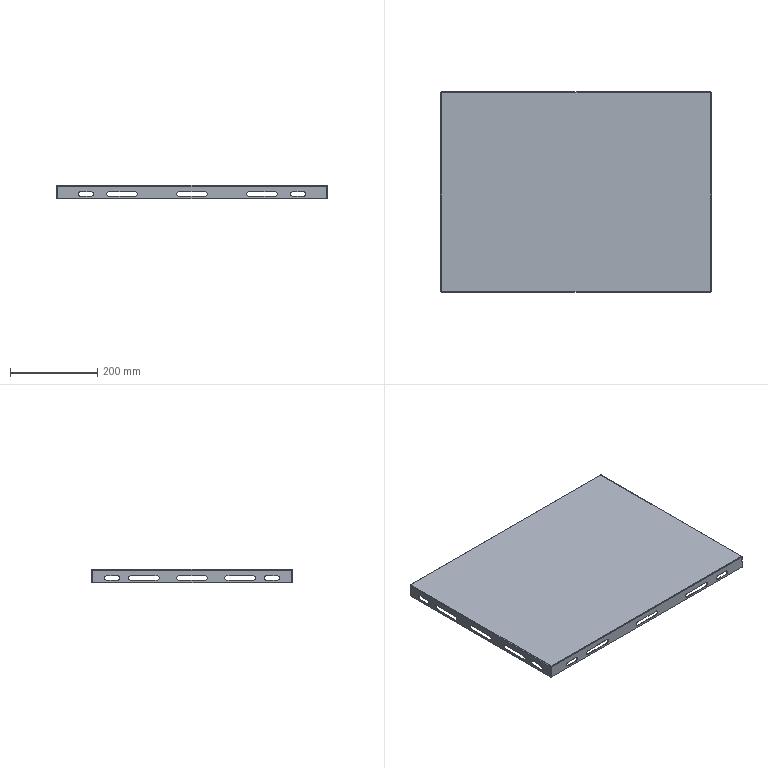Part | SolidWorks | features ICE 2, EdgeFlange 1, FlatPattern 1, SMBaseFlange 1, SheetMetal 1 | 1 solid | 118 faces | box 619 x 459 x 30 mm | volume 499692 mm3 | plane 62 | cylinder 48 | spline 8 | commonest cylinder face diameters 10 x40 1 x4 4 x4